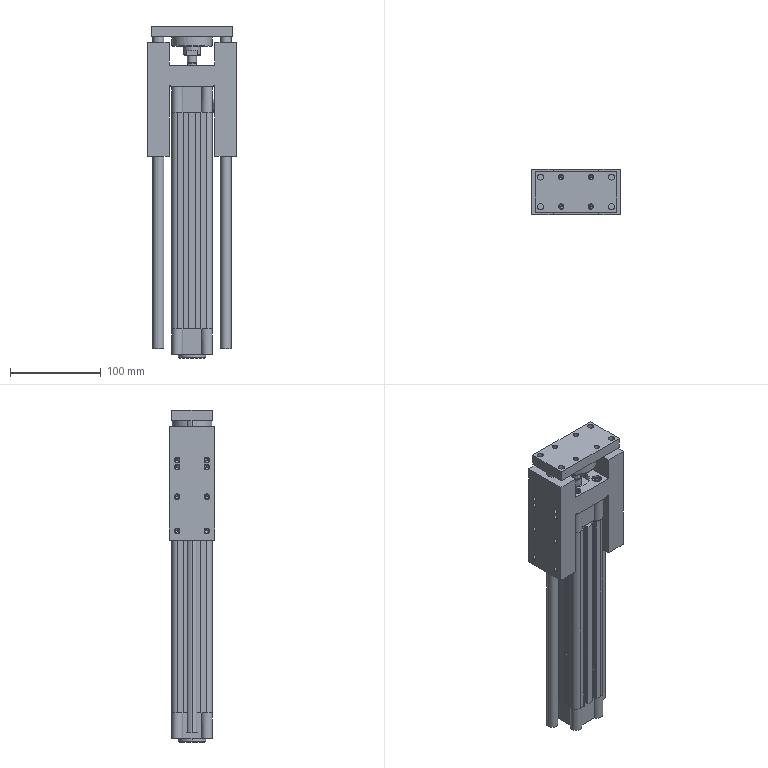Part | STEP file | 535411 DNCI-32-200-P-A-FENG-MS---(asm_0_)(control position cylinder with guide)_5 | 8 solids | 676 faces | box 97 x 50 x 365 mm | volume 831843 mm3 | cylinder 230 | cone 227 | plane 215 | spline 4 | commonest cylinder face diameters 4.917 x56 0.6 x24 0.8 x24 6 x24 6.6 x16 11 x16